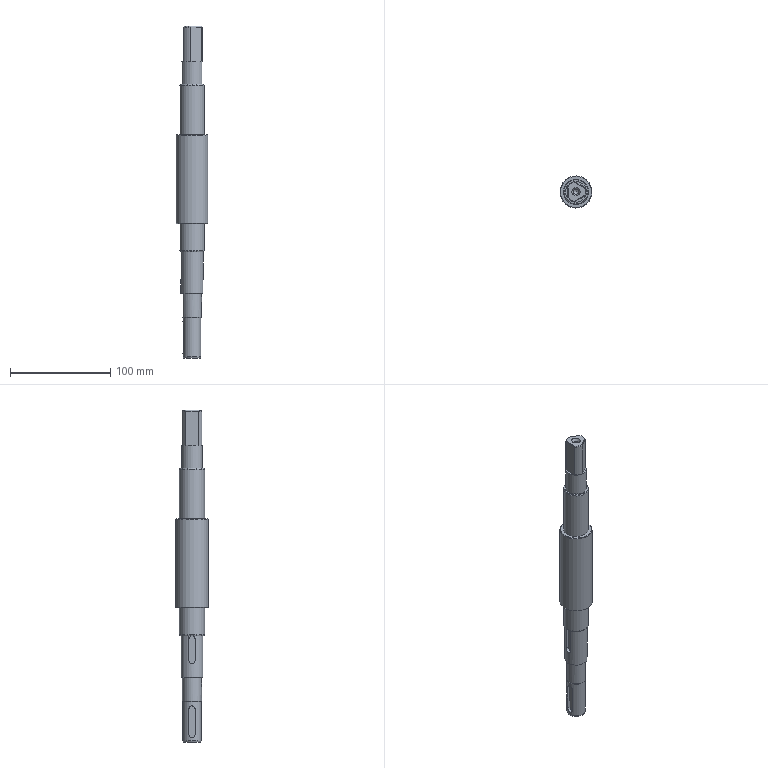NC program | NX | posted with a generic post | part box 32 x 32 x 331.3 mm
Lines 1 to 25 of 3379:
N10 G17 G21 G94 G90
(DRILLING , TOOL : ZXZ)
N12 T01 M6
N14 G54
N16 G17 G0 G90 X-1. Y0. B0. C0. S5000 M3
N18 G43 Z30. H1
N20 G94 G81 G98 Z-1. F250. R3.
N22 G80
N24 G0 X-1. Y0. Z30.
N26 M5
(DRILLING_COPY_COPY_1 , TOOL : 5.0ZT)
N28 T15 M6
N30 G54
N32 G17 G0 G90 X-1. Y0. B0. C0. S2000 M3
N34 G43 Z30. H15
N36 G94 G83 G98 Z-24.502 F150. Q2. R3.
N38 G80
N40 G0 X-1. Y0. Z30.
N42 M5